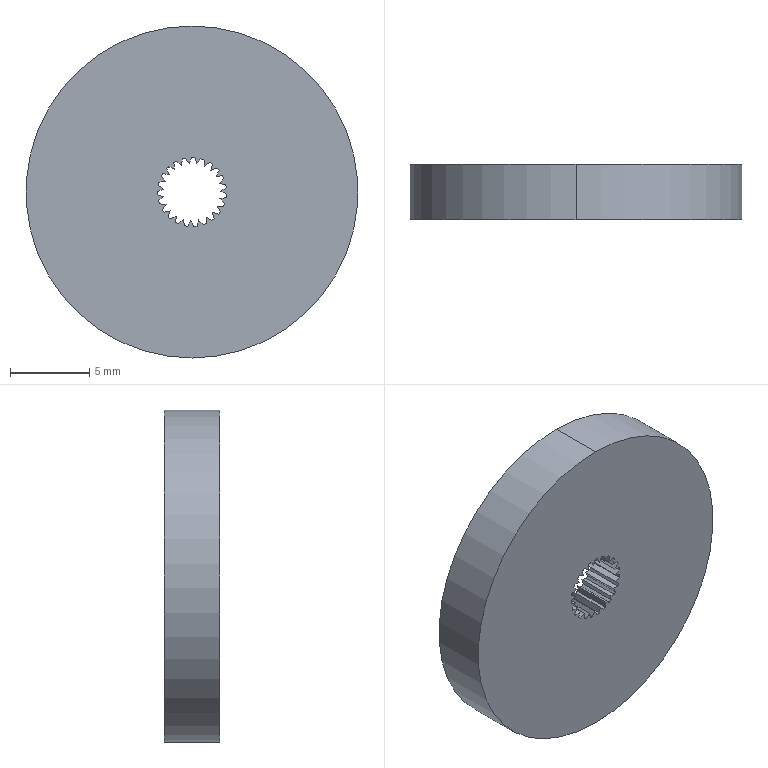Part | SolidWorks | features CombineBodies 1, Extrusion 1, ICE 1, MoveCopyBody 1, Stock 1 | 1 solid | 129 faces | box 21 x 3.5 x 21 mm | volume 1045 mm3 | cylinder 80 | plane 49 | commonest cylinder face diameters 10.8 x28 4.361 x23 11 x14 15 x13 21 x2